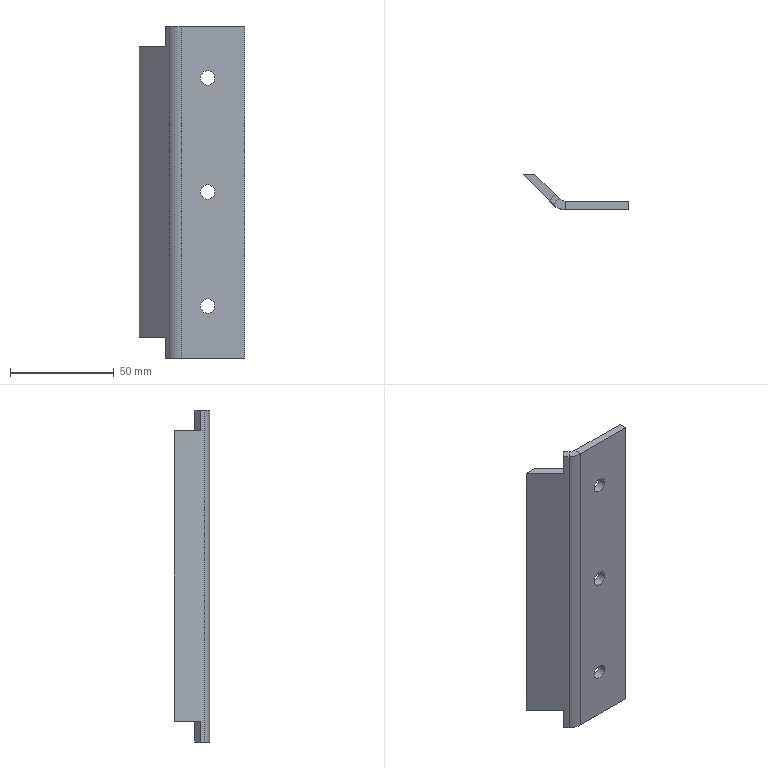Part | SolidWorks | 1 solid | 24 faces | box 51.059 x 17.007 x 160 mm | volume 32939 mm3 | plane 16 | cylinder 8 | commonest cylinder face diameters 7 x6 8 x1 16 x1
STEP:
#1=CARTESIAN_POINT('',(18.5,4.,55.));
#2=VERTEX_POINT('',#1);
#3=CARTESIAN_POINT('',(18.5,0.,55.));
#4=VERTEX_POINT('',#3);
#5=CARTESIAN_POINT('',(18.5,4.,55.));
#6=DIRECTION('',(0.,-1.,0.));
#7=VECTOR('',#6,1000.);
#8=LINE('',#5,#7);
#9=EDGE_CURVE('',#2,#4,#8,.T.);
#10=ORIENTED_EDGE('',*,*,#9,.F.);
#11=CARTESIAN_POINT('',(11.5,4.,55.));
#12=VERTEX_POINT('',#11);
#13=CARTESIAN_POINT('',(15.,4.,55.));
#14=DIRECTION('',(0.,1.,0.));
#15=DIRECTION('',(1.,0.,0.));
#16=AXIS2_PLACEMENT_3D('',#13,#14,#15);
#17=CIRCLE('',#16,3.5);
#18=EDGE_CURVE('',#2,#12,#17,.T.);
#19=ORIENTED_EDGE('',*,*,#18,.T.);
#20=CARTESIAN_POINT('',(11.5,0.,55.));
#21=VERTEX_POINT('',#20);
#22=CARTESIAN_POINT('',(11.5,4.,55.));
#23=DIRECTION('',(0.,-1.,0.));
#24=VECTOR('',#23,1000.);
#25=LINE('',#22,#24);
#26=EDGE_CURVE('',#12,#21,#25,.T.);
#27=ORIENTED_EDGE('',*,*,#26,.T.);
#28=CARTESIAN_POINT('',(15.,0.,55.));
#29=DIRECTION('',(0.,-1.,0.));
#30=DIRECTION('',(-1.,0.,0.));
#31=AXIS2_PLACEMENT_3D('',#28,#29,#30);
#32=CIRCLE('',#31,3.5);
#33=EDGE_CURVE('',#21,#4,#32,.T.);
#34=ORIENTED_EDGE('',*,*,#33,.T.);
#35=EDGE_LOOP('',(#10,#19,#27,#34));
#36=FACE_OUTER_BOUND('',#35,.T.);
#37=CARTESIAN_POINT('',(15.,2.,55.));
#38=DIRECTION('',(0.,1.,0.));
#39=DIRECTION('',(1.,0.,0.));
#40=AXIS2_PLACEMENT_3D('',#37,#38,#39);
#41=CYLINDRICAL_SURFACE('',#40,3.5);
#42=ADVANCED_FACE('',(#36),#41,.F.);
#43=CARTESIAN_POINT('',(15.,4.,55.));
#44=DIRECTION('',(0.,1.,0.));
#45=DIRECTION('',(-1.,0.,0.));
#46=AXIS2_PLACEMENT_3D('',#43,#44,#45);
#47=CIRCLE('',#46,3.5);
#48=EDGE_CURVE('',#12,#2,#47,.T.);
#49=ORIENTED_EDGE('',*,*,#48,.T.);
#50=ORIENTED_EDGE('',*,*,#9,.T.);
#51=CARTESIAN_POINT('',(15.,0.,55.));
#52=DIRECTION('',(0.,-1.,0.));
#53=DIRECTION('',(1.,0.,0.));
#54=AXIS2_PLACEMENT_3D('',#51,#52,#53);
#55=CIRCLE('',#54,3.5);
#56=EDGE_CURVE('',#4,#21,#55,.T.);
#57=ORIENTED_EDGE('',*,*,#56,.T.);
#58=ORIENTED_EDGE('',*,*,#26,.F.);
#59=EDGE_LOOP('',(#49,#50,#57,#58));
#60=FACE_OUTER_BOUND('',#59,.T.);
#61=CARTESIAN_POINT('',(15.,2.,55.));
#62=DIRECTION('',(0.,1.,0.));
#63=DIRECTION('',(1.,0.,0.));
#64=AXIS2_PLACEMENT_3D('',#61,#62,#63);
#65=CYLINDRICAL_SURFACE('',#64,3.5);
#66=ADVANCED_FACE('',(#60),#65,.F.);
#67=CARTESIAN_POINT('',(18.5,4.,-55.));
#68=VERTEX_POINT('',#67);
#69=CARTESIAN_POINT('',(18.5,0.,-55.));
#70=VERTEX_POINT('',#69);
#71=CARTESIAN_POINT('',(18.5,4.,-55.));
#72=DIRECTION('',(0.,-1.,0.));
#73=VECTOR('',#72,1000.);
#74=LINE('',#71,#73);
#75=EDGE_CURVE('',#68,#70,#74,.T.);
#76=ORIENTED_EDGE('',*,*,#75,.F.);
#77=CARTESIAN_POINT('',(11.5,4.,-55.));
#78=VERTEX_POINT('',#77);
#79=CARTESIAN_POINT('',(15.,4.,-55.));
#80=DIRECTION('',(0.,1.,0.));
#81=DIRECTION('',(1.,0.,0.));
#82=AXIS2_PLACEMENT_3D('',#79,#80,#81);
#83=CIRCLE('',#82,3.5);
#84=EDGE_CURVE('',#68,#78,#83,.T.);
#85=ORIENTED_EDGE('',*,*,#84,.T.);
#86=CARTESIAN_POINT('',(11.5,0.,-55.));
#87=VERTEX_POINT('',#86);
#88=CARTESIAN_POINT('',(11.5,4.,-55.));
#89=DIRECTION('',(0.,-1.,0.));
#90=VECTOR('',#89,1000.);
#91=LINE('',#88,#90);
#92=EDGE_CURVE('',#78,#87,#91,.T.);
#93=ORIENTED_EDGE('',*,*,#92,.T.);
#94=CARTESIAN_POINT('',(15.,0.,-55.));
#95=DIRECTION('',(0.,-1.,0.));
#96=DIRECTION('',(-1.,0.,0.));
#97=AXIS2_PLACEMENT_3D('',#94,#95,#96);
#98=CIRCLE('',#97,3.5);
#99=EDGE_CURVE('',#87,#70,#98,.T.);
#100=ORIENTED_EDGE('',*,*,#99,.T.);
#101=EDGE_LOOP('',(#76,#85,#93,#100));
#102=FACE_OUTER_BOUND('',#101,.T.);
#103=CARTESIAN_POINT('',(15.,2.,-55.));
#104=DIRECTION('',(0.,1.,0.));
#105=DIRECTION('',(1.,0.,0.));
#106=AXIS2_PLACEMENT_3D('',#103,#104,#105);
#107=CYLINDRICAL_SURFACE('',#106,3.5);
#108=ADVANCED_FACE('',(#102),#107,.F.);
#109=CARTESIAN_POINT('',(15.,4.,-55.));
#110=DIRECTION('',(0.,1.,0.));
#111=DIRECTION('',(-1.,0.,0.));
#112=AXIS2_PLACEMENT_3D('',#109,#110,#111);
#113=CIRCLE('',#112,3.5);
#114=EDGE_CURVE('',#78,#68,#113,.T.);
#115=ORIENTED_EDGE('',*,*,#114,.T.);
#116=ORIENTED_EDGE('',*,*,#75,.T.);
#117=CARTESIAN_POINT('',(15.,0.,-55.));
#118=DIRECTION('',(0.,-1.,0.));
#119=DIRECTION('',(1.,0.,0.));
#120=AXIS2_PLACEMENT_3D('',#117,#118,#119);
#121=CIRCLE('',#120,3.5);
#122=EDGE_CURVE('',#70,#87,#121,.T.);
#123=ORIENTED_EDGE('',*,*,#122,.T.);
#124=ORIENTED_EDGE('',*,*,#92,.F.);
#125=EDGE_LOOP('',(#115,#116,#123,#124));
#126=FACE_OUTER_BOUND('',#125,.T.);
#127=CARTESIAN_POINT('',(15.,2.,-55.));
#128=DIRECTION('',(0.,1.,0.));
#129=DIRECTION('',(1.,0.,0.));
#130=AXIS2_PLACEMENT_3D('',#127,#128,#129);
#131=CYLINDRICAL_SURFACE('',#130,3.5);
#132=ADVANCED_FACE('',(#126),#131,.F.);
#133=CARTESIAN_POINT('',(18.5,4.,0.));
#134=VERTEX_POINT('',#133);
#135=CARTESIAN_POINT('',(18.5,0.,0.));
#136=VERTEX_POINT('',#135);
#137=CARTESIAN_POINT('',(18.5,4.,0.));
#138=DIRECTION('',(0.,-1.,0.));
#139=VECTOR('',#138,1000.);
#140=LINE('',#137,#139);
#141=EDGE_CURVE('',#134,#136,#140,.T.);
#142=ORIENTED_EDGE('',*,*,#141,.F.);
#143=CARTESIAN_POINT('',(11.5,4.,0.));
#144=VERTEX_POINT('',#143);
#145=CARTESIAN_POINT('',(15.,4.,0.));
#146=DIRECTION('',(0.,1.,0.));
#147=DIRECTION('',(1.,0.,0.));
#148=AXIS2_PLACEMENT_3D('',#145,#146,#147);
#149=CIRCLE('',#148,3.5);
#150=EDGE_CURVE('',#134,#144,#149,.T.);
#151=ORIENTED_EDGE('',*,*,#150,.T.);
#152=CARTESIAN_POINT('',(11.5,0.,0.));
#153=VERTEX_POINT('',#152);
#154=CARTESIAN_POINT('',(11.5,4.,0.));
#155=DIRECTION('',(0.,-1.,0.));
#156=VECTOR('',#155,1000.);
#157=LINE('',#154,#156);
#158=EDGE_CURVE('',#144,#153,#157,.T.);
#159=ORIENTED_EDGE('',*,*,#158,.T.);
#160=CARTESIAN_POINT('',(15.,0.,0.));
#161=DIRECTION('',(0.,-1.,0.));
#162=DIRECTION('',(-1.,0.,0.));
#163=AXIS2_PLACEMENT_3D('',#160,#161,#162);
#164=CIRCLE('',#163,3.5);
#165=EDGE_CURVE('',#153,#136,#164,.T.);
#166=ORIENTED_EDGE('',*,*,#165,.T.);
#167=EDGE_LOOP('',(#142,#151,#159,#166));
#168=FACE_OUTER_BOUND('',#167,.T.);
#169=CARTESIAN_POINT('',(15.,2.,0.));
#170=DIRECTION('',(0.,1.,0.));
#171=DIRECTION('',(1.,0.,0.));
#172=AXIS2_PLACEMENT_3D('',#169,#170,#171);
#173=CYLINDRICAL_SURFACE('',#172,3.5);
#174=ADVANCED_FACE('',(#168),#173,.F.);
#175=CARTESIAN_POINT('',(15.,4.,0.));
#176=DIRECTION('',(0.,1.,0.));
#177=DIRECTION('',(-1.,0.,0.));
#178=AXIS2_PLACEMENT_3D('',#175,#176,#177);
#179=CIRCLE('',#178,3.5);
#180=EDGE_CURVE('',#144,#134,#179,.T.);
#181=ORIENTED_EDGE('',*,*,#180,.T.);
#182=ORIENTED_EDGE('',*,*,#141,.T.);
#183=CARTESIAN_POINT('',(15.,0.,0.));
#184=DIRECTION('',(0.,-1.,0.));
#185=DIRECTION('',(1.,0.,0.));
#186=AXIS2_PLACEMENT_3D('',#183,#184,#185);
#187=CIRCLE('',#186,3.5);
#188=EDGE_CURVE('',#136,#153,#187,.T.);
#189=ORIENTED_EDGE('',*,*,#188,.T.);
#190=ORIENTED_EDGE('',*,*,#158,.F.);
#191=EDGE_LOOP('',(#181,#182,#189,#190));
#192=FACE_OUTER_BOUND('',#191,.T.);
#193=CARTESIAN_POINT('',(15.,2.,0.));
#194=DIRECTION('',(0.,1.,0.));
#195=DIRECTION('',(1.,0.,0.));
#196=AXIS2_PLACEMENT_3D('',#193,#194,#195);
#197=CYLINDRICAL_SURFACE('',#196,3.5);
#198=ADVANCED_FACE('',(#192),#197,.F.);
#199=CARTESIAN_POINT('',(33.,4.,-80.));
#200=VERTEX_POINT('',#199);
#201=CARTESIAN_POINT('',(33.,4.,80.));
#202=VERTEX_POINT('',#201);
#203=CARTESIAN_POINT('',(33.,4.,-80.));
#204=DIRECTION('',(0.,0.,1.));
#205=VECTOR('',#204,1000.);
#206=LINE('',#203,#205);
#207=EDGE_CURVE('',#200,#202,#206,.T.);
#208=ORIENTED_EDGE('',*,*,#207,.T.);
#209=CARTESIAN_POINT('',(33.,0.,80.));
#210=VERTEX_POINT('',#209);
#211=CARTESIAN_POINT('',(33.,0.,80.));
#212=DIRECTION('',(0.,1.,0.));
#213=VECTOR('',#212,1000.);
#214=LINE('',#211,#213);
#215=EDGE_CURVE('',#210,#202,#214,.T.);
#216=ORIENTED_EDGE('',*,*,#215,.F.);
#217=CARTESIAN_POINT('',(33.,0.,-80.));
#218=VERTEX_POINT('',#217);
#219=CARTESIAN_POINT('',(33.,0.,-80.));
#220=DIRECTION('',(0.,0.,1.));
#221=VECTOR('',#220,1000.);
#222=LINE('',#219,#221);
#223=EDGE_CURVE('',#218,#210,#222,.T.);
#224=ORIENTED_EDGE('',*,*,#223,.F.);
#225=CARTESIAN_POINT('',(33.,0.,-80.));
#226=DIRECTION('',(0.,1.,0.));
#227=VECTOR('',#226,1000.);
#228=LINE('',#225,#227);
#229=EDGE_CURVE('',#218,#200,#228,.T.);
#230=ORIENTED_EDGE('',*,*,#229,.T.);
#231=EDGE_LOOP('',(#208,#216,#224,#230));
#232=FACE_OUTER_BOUND('',#231,.T.);
#233=CARTESIAN_POINT('',(33.,4.,80.));
#234=DIRECTION('',(1.,0.,0.));
#235=DIRECTION('',(0.,1.,0.));
#236=AXIS2_PLACEMENT_3D('',#233,#234,#235);
#237=PLANE('',#236);
#238=ADVANCED_FACE('',(#232),#237,.T.);
#239=CARTESIAN_POINT('',(-2.503,7.108,70.));
#240=VERTEX_POINT('',#239);
#241=CARTESIAN_POINT('',(-5.331,4.279,70.));
#242=VERTEX_POINT('',#241);
#243=CARTESIAN_POINT('',(-2.503,7.108,70.));
#244=DIRECTION('',(-0.7071,-0.7071,0.));
#245=VECTOR('',#244,1000.);
#246=LINE('',#243,#245);
#247=EDGE_CURVE('',#240,#242,#246,.T.);
#248=ORIENTED_EDGE('',*,*,#247,.F.);
#249=CARTESIAN_POINT('',(-12.402,17.007,70.));
#250=VERTEX_POINT('',#249);
#251=CARTESIAN_POINT('',(-12.402,17.007,70.));
#252=DIRECTION('',(0.7071,-0.7071,0.));
#253=VECTOR('',#252,1000.);
#254=LINE('',#251,#253);
#255=EDGE_CURVE('',#250,#240,#254,.T.);
#256=ORIENTED_EDGE('',*,*,#255,.F.);
#257=CARTESIAN_POINT('',(-18.059,17.007,70.));
#258=VERTEX_POINT('',#257);
#259=CARTESIAN_POINT('',(-12.402,17.007,70.));
#260=DIRECTION('',(-1.,0.,0.));
#261=VECTOR('',#260,1000.);
#262=LINE('',#259,#261);
#263=EDGE_CURVE('',#250,#258,#262,.T.);
#264=ORIENTED_EDGE('',*,*,#263,.T.);
#265=CARTESIAN_POINT('',(-5.331,4.279,70.));
#266=DIRECTION('',(-0.7071,0.7071,0.));
#267=VECTOR('',#266,1000.);
#268=LINE('',#265,#267);
#269=EDGE_CURVE('',#242,#258,#268,.T.);
#270=ORIENTED_EDGE('',*,*,#269,.F.);
#271=EDGE_LOOP('',(#248,#256,#264,#270));
#272=FACE_OUTER_BOUND('',#271,.T.);
#273=CARTESIAN_POINT('',(-15.23,19.836,70.));
#274=DIRECTION('',(0.,0.,-1.));
#275=DIRECTION('',(0.,-1.,0.));
#276=AXIS2_PLACEMENT_3D('',#273,#274,#275);
#277=PLANE('',#276);
#278=ADVANCED_FACE('',(#272),#277,.F.);
#279=CARTESIAN_POINT('',(-5.331,4.279,80.));
#280=VERTEX_POINT('',#279);
#281=CARTESIAN_POINT('',(-5.331,4.279,70.));
#282=DIRECTION('',(0.,0.,1.));
#283=VECTOR('',#282,1000.);
#284=LINE('',#281,#283);
#285=EDGE_CURVE('',#242,#280,#284,.T.);
#286=ORIENTED_EDGE('',*,*,#285,.T.);
#287=CARTESIAN_POINT('',(-2.503,7.108,80.));
#288=VERTEX_POINT('',#287);
#289=CARTESIAN_POINT('',(-5.331,4.279,80.));
#290=DIRECTION('',(0.7071,0.7071,0.));
#291=VECTOR('',#290,1000.);
#292=LINE('',#289,#291);
#293=EDGE_CURVE('',#280,#288,#292,.T.);
#294=ORIENTED_EDGE('',*,*,#293,.T.);
#295=CARTESIAN_POINT('',(-2.503,7.108,80.));
#296=DIRECTION('',(0.,0.,-1.));
#297=VECTOR('',#296,1000.);
#298=LINE('',#295,#297);
#299=EDGE_CURVE('',#288,#240,#298,.T.);
#300=ORIENTED_EDGE('',*,*,#299,.T.);
#301=ORIENTED_EDGE('',*,*,#247,.T.);
#302=EDGE_LOOP('',(#286,#294,#300,#301));
#303=FACE_OUTER_BOUND('',#302,.T.);
#304=CARTESIAN_POINT('',(-2.503,7.108,70.));
#305=DIRECTION('',(0.7071,-0.7071,0.));
#306=DIRECTION('',(0.,0.,-1.));
#307=AXIS2_PLACEMENT_3D('',#304,#305,#306);
#308=PLANE('',#307);
#309=ADVANCED_FACE('',(#303),#308,.F.);
#310=CARTESIAN_POINT('',(-3.395,2.343,-80.));
#311=VERTEX_POINT('',#310);
#312=CARTESIAN_POINT('',(2.262,0.,-80.));
#313=VERTEX_POINT('',#312);
#314=CARTESIAN_POINT('',(2.262,8.,-80.));
#315=DIRECTION('',(0.,0.,1.));
#316=DIRECTION('',(-0.7071,-0.7071,0.));
#317=AXIS2_PLACEMENT_3D('',#314,#315,#316);
#318=CIRCLE('',#317,8.);
#319=EDGE_CURVE('',#311,#313,#318,.T.);
#320=ORIENTED_EDGE('',*,*,#319,.T.);
#321=CARTESIAN_POINT('',(2.262,0.,80.));
#322=VERTEX_POINT('',#321);
#323=CARTESIAN_POINT('',(2.262,0.,80.));
#324=DIRECTION('',(0.,0.,-1.));
#325=VECTOR('',#324,1000.);
#326=LINE('',#323,#325);
#327=EDGE_CURVE('',#322,#313,#326,.T.);
#328=ORIENTED_EDGE('',*,*,#327,.F.);
#329=CARTESIAN_POINT('',(-3.395,2.343,80.));
#330=VERTEX_POINT('',#329);
#331=CARTESIAN_POINT('',(2.262,8.,80.));
#332=DIRECTION('',(0.,0.,-1.));
#333=DIRECTION('',(0.,-1.,0.));
#334=AXIS2_PLACEMENT_3D('',#331,#332,#333);
#335=CIRCLE('',#334,8.);
#336=EDGE_CURVE('',#322,#330,#335,.T.);
#337=ORIENTED_EDGE('',*,*,#336,.T.);
#338=CARTESIAN_POINT('',(-3.395,2.343,-80.));
#339=DIRECTION('',(0.,0.,1.));
#340=VECTOR('',#339,1000.);
#341=LINE('',#338,#340);
#342=EDGE_CURVE('',#311,#330,#341,.T.);
#343=ORIENTED_EDGE('',*,*,#342,.F.);
#344=EDGE_LOOP('',(#320,#328,#337,#343));
#345=FACE_OUTER_BOUND('',#344,.T.);
#346=CARTESIAN_POINT('',(2.262,8.,0.));
#347=DIRECTION('',(0.,0.,-1.));
#348=DIRECTION('',(0.,-1.,0.));
#349=AXIS2_PLACEMENT_3D('',#346,#347,#348);
#350=CYLINDRICAL_SURFACE('',#349,8.);
#351=ADVANCED_FACE('',(#345),#350,.T.);
#352=CARTESIAN_POINT('',(-0.5665,5.172,80.));
#353=VERTEX_POINT('',#352);
#354=CARTESIAN_POINT('',(2.262,4.,80.));
#355=VERTEX_POINT('',#354);
#356=CARTESIAN_POINT('',(2.262,8.,80.));
#357=DIRECTION('',(0.,0.,1.));
#358=DIRECTION('',(-0.7071,-0.7071,0.));
#359=AXIS2_PLACEMENT_3D('',#356,#357,#358);
#360=CIRCLE('',#359,4.);
#361=EDGE_CURVE('',#353,#355,#360,.T.);
#362=ORIENTED_EDGE('',*,*,#361,.F.);
#363=CARTESIAN_POINT('',(-0.5665,5.172,80.));
#364=DIRECTION('',(-0.7071,-0.7071,0.));
#365=VECTOR('',#364,1000.);
#366=LINE('',#363,#365);
#367=EDGE_CURVE('',#353,#330,#366,.T.);
#368=ORIENTED_EDGE('',*,*,#367,.T.);
#369=ORIENTED_EDGE('',*,*,#336,.F.);
#370=CARTESIAN_POINT('',(2.262,0.,80.));
#371=DIRECTION('',(0.,1.,0.));
#372=VECTOR('',#371,1000.);
#373=LINE('',#370,#372);
#374=EDGE_CURVE('',#322,#355,#373,.T.);
#375=ORIENTED_EDGE('',*,*,#374,.T.);
#376=EDGE_LOOP('',(#362,#368,#369,#375));
#377=FACE_OUTER_BOUND('',#376,.T.);
#378=CARTESIAN_POINT('',(2.262,-7.,80.));
#379=DIRECTION('',(0.,0.,-1.));
#380=DIRECTION('',(0.,-1.,0.));
#381=AXIS2_PLACEMENT_3D('',#378,#379,#380);
#382=PLANE('',#381);
#383=ADVANCED_FACE('',(#377),#382,.F.);
#384=ORIENTED_EDGE('',*,*,#293,.F.);
#385=CARTESIAN_POINT('',(-3.395,2.343,80.));
#386=DIRECTION('',(-0.7071,0.7071,0.));
#387=VECTOR('',#386,1000.);
#388=LINE('',#385,#387);
#389=EDGE_CURVE('',#330,#280,#388,.T.);
#390=ORIENTED_EDGE('',*,*,#389,.F.);
#391=ORIENTED_EDGE('',*,*,#367,.F.);
#392=CARTESIAN_POINT('',(-2.503,7.108,80.));
#393=DIRECTION('',(0.7071,-0.7071,0.));
#394=VECTOR('',#393,1000.);
#395=LINE('',#392,#394);
#396=EDGE_CURVE('',#288,#353,#395,.T.);
#397=ORIENTED_EDGE('',*,*,#396,.F.);
#398=EDGE_LOOP('',(#384,#390,#391,#397));
#399=FACE_OUTER_BOUND('',#398,.T.);
#400=CARTESIAN_POINT('',(14.468,-15.52,80.));
#401=DIRECTION('',(0.,0.,1.));
#402=DIRECTION('',(1.,0.,0.));
#403=AXIS2_PLACEMENT_3D('',#400,#401,#402);
#404=PLANE('',#403);
#405=ADVANCED_FACE('',(#399),#404,.T.);
#406=CARTESIAN_POINT('',(-5.331,4.279,-80.));
#407=VERTEX_POINT('',#406);
#408=CARTESIAN_POINT('',(-5.331,4.279,-70.));
#409=VERTEX_POINT('',#408);
#410=CARTESIAN_POINT('',(-5.331,4.279,-80.));
#411=DIRECTION('',(0.,0.,1.));
#412=VECTOR('',#411,1000.);
#413=LINE('',#410,#412);
#414=EDGE_CURVE('',#407,#409,#413,.T.);
#415=ORIENTED_EDGE('',*,*,#414,.T.);
#416=CARTESIAN_POINT('',(-2.503,7.108,-70.));
#417=VERTEX_POINT('',#416);
#418=CARTESIAN_POINT('',(-5.331,4.279,-70.));
#419=DIRECTION('',(0.7071,0.7071,0.));
#420=VECTOR('',#419,1000.);
#421=LINE('',#418,#420);
#422=EDGE_CURVE('',#409,#417,#421,.T.);
#423=ORIENTED_EDGE('',*,*,#422,.T.);
#424=CARTESIAN_POINT('',(-2.503,7.108,-80.));
#425=VERTEX_POINT('',#424);
#426=CARTESIAN_POINT('',(-2.503,7.108,-70.));
#427=DIRECTION('',(0.,0.,-1.));
#428=VECTOR('',#427,1000.);
#429=LINE('',#426,#428);
#430=EDGE_CURVE('',#417,#425,#429,.T.);
#431=ORIENTED_EDGE('',*,*,#430,.T.);
#432=CARTESIAN_POINT('',(-2.503,7.108,-80.));
#433=DIRECTION('',(-0.7071,-0.7071,0.));
#434=VECTOR('',#433,1000.);
#435=LINE('',#432,#434);
#436=EDGE_CURVE('',#425,#407,#435,.T.);
#437=ORIENTED_EDGE('',*,*,#436,.T.);
#438=EDGE_LOOP('',(#415,#423,#431,#437));
#439=FACE_OUTER_BOUND('',#438,.T.);
#440=CARTESIAN_POINT('',(-2.503,7.108,-80.));
#441=DIRECTION('',(0.7071,-0.7071,0.));
#442=DIRECTION('',(0.,0.,-1.));
#443=AXIS2_PLACEMENT_3D('',#440,#441,#442);
#444=PLANE('',#443);
#445=ADVANCED_FACE('',(#439),#444,.F.);
#446=ORIENTED_EDGE('',*,*,#255,.T.);
#447=ORIENTED_EDGE('',*,*,#299,.F.);
#448=ORIENTED_EDGE('',*,*,#396,.T.);
#449=CARTESIAN_POINT('',(-0.5665,5.172,-80.));
#450=VERTEX_POINT('',#449);
#451=CARTESIAN_POINT('',(-0.5665,5.172,80.));
#452=DIRECTION('',(0.,0.,-1.));
#453=VECTOR('',#452,1000.);
#454=LINE('',#451,#453);
#455=EDGE_CURVE('',#353,#450,#454,.T.);
#456=ORIENTED_EDGE('',*,*,#455,.T.);
#457=CARTESIAN_POINT('',(-0.5665,5.172,-80.));
#458=DIRECTION('',(-0.7071,0.7071,0.));
#459=VECTOR('',#458,1000.);
#460=LINE('',#457,#459);
#461=EDGE_CURVE('',#450,#425,#460,.T.);
#462=ORIENTED_EDGE('',*,*,#461,.T.);
#463=ORIENTED_EDGE('',*,*,#430,.F.);
#464=CARTESIAN_POINT('',(-12.402,17.007,-70.));
#465=VERTEX_POINT('',#464);
#466=CARTESIAN_POINT('',(-2.503,7.108,-70.));
#467=DIRECTION('',(-0.7071,0.7071,0.));
#468=VECTOR('',#467,1000.);
#469=LINE('',#466,#468);
#470=EDGE_CURVE('',#417,#465,#469,.T.);
#471=ORIENTED_EDGE('',*,*,#470,.T.);
#472=CARTESIAN_POINT('',(-12.402,17.007,-70.));
#473=DIRECTION('',(0.,0.,1.));
#474=VECTOR('',#473,1000.);
#475=LINE('',#472,#474);
#476=EDGE_CURVE('',#465,#250,#475,.T.);
#477=ORIENTED_EDGE('',*,*,#476,.T.);
#478=EDGE_LOOP('',(#446,#447,#448,#456,#462,#463,#471,#477));
#479=FACE_OUTER_BOUND('',#478,.T.);
#480=CARTESIAN_POINT('',(1.033,3.572,0.));
#481=DIRECTION('',(0.7071,0.7071,0.));
#482=DIRECTION('',(0.,0.,-1.));
#483=AXIS2_PLACEMENT_3D('',#480,#481,#482);
#484=PLANE('',#483);
#485=ADVANCED_FACE('',(#479),#484,.T.);
#486=ORIENTED_EDGE('',*,*,#422,.F.);
#487=CARTESIAN_POINT('',(-18.059,17.007,-70.));
#488=VERTEX_POINT('',#487);
#489=CARTESIAN_POINT('',(-18.059,17.007,-70.));
#490=DIRECTION('',(0.7071,-0.7071,0.));
#491=VECTOR('',#490,1000.);
#492=LINE('',#489,#491);
#493=EDGE_CURVE('',#488,#409,#492,.T.);
#494=ORIENTED_EDGE('',*,*,#493,.F.);
#495=CARTESIAN_POINT('',(-18.059,17.007,-70.));
#496=DIRECTION('',(1.,0.,0.));
#497=VECTOR('',#496,1000.);
#498=LINE('',#495,#497);
#499=EDGE_CURVE('',#488,#465,#498,.T.);
#500=ORIENTED_EDGE('',*,*,#499,.T.);
#501=ORIENTED_EDGE('',*,*,#470,.F.);
#502=EDGE_LOOP('',(#486,#494,#500,#501));
#503=FACE_OUTER_BOUND('',#502,.T.);
#504=CARTESIAN_POINT('',(-2.503,7.108,-70.));
#505=DIRECTION('',(0.,0.,1.));
#506=DIRECTION('',(1.,0.,0.));
#507=AXIS2_PLACEMENT_3D('',#504,#505,#506);
#508=PLANE('',#507);
#509=ADVANCED_FACE('',(#503),#508,.F.);
#510=ORIENTED_EDGE('',*,*,#263,.F.);
#511=ORIENTED_EDGE('',*,*,#476,.F.);
#512=ORIENTED_EDGE('',*,*,#499,.F.);
#513=CARTESIAN_POINT('',(-18.059,17.007,70.));
#514=DIRECTION('',(0.,0.,-1.));
#515=VECTOR('',#514,1000.);
#516=LINE('',#513,#515);
#517=EDGE_CURVE('',#258,#488,#516,.T.);
#518=ORIENTED_EDGE('',*,*,#517,.F.);
#519=EDGE_LOOP('',(#510,#511,#512,#518));
#520=FACE_OUTER_BOUND('',#519,.T.);
#521=CARTESIAN_POINT('',(-15.23,17.007,40.));
#522=DIRECTION('',(0.,1.,0.));
#523=DIRECTION('',(1.,0.,0.));
#524=AXIS2_PLACEMENT_3D('',#521,#522,#523);
#525=PLANE('',#524);
#526=ADVANCED_FACE('',(#520),#525,.T.);
#527=ORIENTED_EDGE('',*,*,#493,.T.);
#528=ORIENTED_EDGE('',*,*,#414,.F.);
#529=CARTESIAN_POINT('',(-5.331,4.279,-80.));
#530=DIRECTION('',(0.7071,-0.7071,0.));
#531=VECTOR('',#530,1000.);
#532=LINE('',#529,#531);
#533=EDGE_CURVE('',#407,#311,#532,.T.);
#534=ORIENTED_EDGE('',*,*,#533,.T.);
#535=ORIENTED_EDGE('',*,*,#342,.T.);
#536=ORIENTED_EDGE('',*,*,#389,.T.);
#537=ORIENTED_EDGE('',*,*,#285,.F.);
#538=ORIENTED_EDGE('',*,*,#269,.T.);
#539=ORIENTED_EDGE('',*,*,#517,.T.);
#540=EDGE_LOOP('',(#527,#528,#534,#535,#536,#537,#538,#539));
#541=FACE_OUTER_BOUND('',#540,.T.);
#542=CARTESIAN_POINT('',(-1.795,0.7437,0.));
#543=DIRECTION('',(0.7071,0.7071,0.));
#544=DIRECTION('',(0.,0.,-1.));
#545=AXIS2_PLACEMENT_3D('',#542,#543,#544);
#546=PLANE('',#545);
#547=ADVANCED_FACE('',(#541),#546,.F.);
#548=ORIENTED_EDGE('',*,*,#436,.F.);
#549=ORIENTED_EDGE('',*,*,#461,.F.);
#550=CARTESIAN_POINT('',(-3.395,2.343,-80.));
#551=DIRECTION('',(0.7071,0.7071,0.));
#552=VECTOR('',#551,1000.);
#553=LINE('',#550,#552);
#554=EDGE_CURVE('',#311,#450,#553,.T.);
#555=ORIENTED_EDGE('',*,*,#554,.F.);
#556=ORIENTED_EDGE('',*,*,#533,.F.);
#557=EDGE_LOOP('',(#548,#549,#555,#556));
#558=FACE_OUTER_BOUND('',#557,.T.);
#559=CARTESIAN_POINT('',(-18.059,17.007,-80.));
#560=DIRECTION('',(0.,0.,-1.));
#561=DIRECTION('',(0.,-1.,0.));
#562=AXIS2_PLACEMENT_3D('',#559,#560,#561);
#563=PLANE('',#562);
#564=ADVANCED_FACE('',(#558),#563,.T.);
#565=CARTESIAN_POINT('',(2.262,4.,-80.));
#566=VERTEX_POINT('',#565);
#567=CARTESIAN_POINT('',(2.262,8.,-80.));
#568=DIRECTION('',(0.,0.,-1.));
#569=DIRECTION('',(0.,-1.,0.));
#570=AXIS2_PLACEMENT_3D('',#567,#568,#569);
#571=CIRCLE('',#570,4.);
#572=EDGE_CURVE('',#566,#450,#571,.T.);
#573=ORIENTED_EDGE('',*,*,#572,.F.);
#574=CARTESIAN_POINT('',(2.262,4.,-80.));
#575=DIRECTION('',(0.,-1.,0.));
#576=VECTOR('',#575,1000.);
#577=LINE('',#574,#576);
#578=EDGE_CURVE('',#566,#313,#577,.T.);
#579=ORIENTED_EDGE('',*,*,#578,.T.);
#580=ORIENTED_EDGE('',*,*,#319,.F.);
#581=ORIENTED_EDGE('',*,*,#554,.T.);
#582=EDGE_LOOP('',(#573,#579,#580,#581));
#583=FACE_OUTER_BOUND('',#582,.T.);
#584=CARTESIAN_POINT('',(2.262,-7.,-80.));
#585=DIRECTION('',(0.,0.,-1.));
#586=DIRECTION('',(0.,-1.,0.));
#587=AXIS2_PLACEMENT_3D('',#584,#585,#586);
#588=PLANE('',#587);
#589=ADVANCED_FACE('',(#583),#588,.T.);
#590=ORIENTED_EDGE('',*,*,#229,.F.);
#591=CARTESIAN_POINT('',(33.,0.,-80.));
#592=DIRECTION('',(-1.,0.,0.));
#593=VECTOR('',#592,1000.);
#594=LINE('',#591,#593);
#595=EDGE_CURVE('',#218,#313,#594,.T.);
#596=ORIENTED_EDGE('',*,*,#595,.T.);
#597=ORIENTED_EDGE('',*,*,#578,.F.);
#598=CARTESIAN_POINT('',(2.262,4.,-80.));
#599=DIRECTION('',(1.,0.,0.));
#600=VECTOR('',#599,1000.);
#601=LINE('',#598,#600);
#602=EDGE_CURVE('',#566,#200,#601,.T.);
#603=ORIENTED_EDGE('',*,*,#602,.T.);
#604=EDGE_LOOP('',(#590,#596,#597,#603));
#605=FACE_OUTER_BOUND('',#604,.T.);
#606=CARTESIAN_POINT('',(-23.,0.,-80.));
#607=DIRECTION('',(0.,0.,-1.));
#608=DIRECTION('',(0.,-1.,0.));
#609=AXIS2_PLACEMENT_3D('',#606,#607,#608);
#610=PLANE('',#609);
#611=ADVANCED_FACE('',(#605),#610,.T.);
#612=ORIENTED_EDGE('',*,*,#33,.F.);
#613=ORIENTED_EDGE('',*,*,#56,.F.);
#614=EDGE_LOOP('',(#612,#613));
#615=FACE_BOUND('',#614,.T.);
#616=ORIENTED_EDGE('',*,*,#99,.F.);
#617=ORIENTED_EDGE('',*,*,#122,.F.);
#618=EDGE_LOOP('',(#616,#617));
#619=FACE_BOUND('',#618,.T.);
#620=ORIENTED_EDGE('',*,*,#165,.F.);
#621=ORIENTED_EDGE('',*,*,#188,.F.);
#622=EDGE_LOOP('',(#620,#621));
#623=FACE_BOUND('',#622,.T.);
#624=ORIENTED_EDGE('',*,*,#223,.T.);
#625=CARTESIAN_POINT('',(2.262,0.,80.));
#626=DIRECTION('',(1.,0.,0.));
#627=VECTOR('',#626,1000.);
#628=LINE('',#625,#627);
#629=EDGE_CURVE('',#322,#210,#628,.T.);
#630=ORIENTED_EDGE('',*,*,#629,.F.);
#631=ORIENTED_EDGE('',*,*,#327,.T.);
#632=ORIENTED_EDGE('',*,*,#595,.F.);
#633=EDGE_LOOP('',(#624,#630,#631,#632));
#634=FACE_OUTER_BOUND('',#633,.T.);
#635=CARTESIAN_POINT('',(0.,0.,0.));
#636=DIRECTION('',(0.,1.,0.));
#637=DIRECTION('',(1.,0.,0.));
#638=AXIS2_PLACEMENT_3D('',#635,#636,#637);
#639=PLANE('',#638);
#640=ADVANCED_FACE('',(#615,#619,#623,#634),#639,.F.);
#641=ORIENTED_EDGE('',*,*,#215,.T.);
#642=CARTESIAN_POINT('',(2.262,4.,80.));
#643=DIRECTION('',(1.,0.,0.));
#644=VECTOR('',#643,1000.);
#645=LINE('',#642,#644);
#646=EDGE_CURVE('',#355,#202,#645,.T.);
#647=ORIENTED_EDGE('',*,*,#646,.F.);
#648=ORIENTED_EDGE('',*,*,#374,.F.);
#649=ORIENTED_EDGE('',*,*,#629,.T.);
#650=EDGE_LOOP('',(#641,#647,#648,#649));
#651=FACE_OUTER_BOUND('',#650,.T.);
#652=CARTESIAN_POINT('',(23.,0.,80.));
#653=DIRECTION('',(0.,0.,1.));
#654=DIRECTION('',(1.,0.,0.));
#655=AXIS2_PLACEMENT_3D('',#652,#653,#654);
#656=PLANE('',#655);
#657=ADVANCED_FACE('',(#651),#656,.T.);
#658=ORIENTED_EDGE('',*,*,#48,.F.);
#659=ORIENTED_EDGE('',*,*,#18,.F.);
#660=EDGE_LOOP('',(#658,#659));
#661=FACE_BOUND('',#660,.T.);
#662=ORIENTED_EDGE('',*,*,#114,.F.);
#663=ORIENTED_EDGE('',*,*,#84,.F.);
#664=EDGE_LOOP('',(#662,#663));
#665=FACE_BOUND('',#664,.T.);
#666=ORIENTED_EDGE('',*,*,#180,.F.);
#667=ORIENTED_EDGE('',*,*,#150,.F.);
#668=EDGE_LOOP('',(#666,#667));
#669=FACE_BOUND('',#668,.T.);
#670=ORIENTED_EDGE('',*,*,#207,.F.);
#671=ORIENTED_EDGE('',*,*,#602,.F.);
#672=CARTESIAN_POINT('',(2.262,4.,-80.));
#673=DIRECTION('',(0.,0.,1.));
#674=VECTOR('',#673,1000.);
#675=LINE('',#672,#674);
#676=EDGE_CURVE('',#566,#355,#675,.T.);
#677=ORIENTED_EDGE('',*,*,#676,.T.);
#678=ORIENTED_EDGE('',*,*,#646,.T.);
#679=EDGE_LOOP('',(#670,#671,#677,#678));
#680=FACE_OUTER_BOUND('',#679,.T.);
#681=CARTESIAN_POINT('',(0.,4.,0.));
#682=DIRECTION('',(0.,1.,0.));
#683=DIRECTION('',(1.,0.,0.));
#684=AXIS2_PLACEMENT_3D('',#681,#682,#683);
#685=PLANE('',#684);
#686=ADVANCED_FACE('',(#661,#665,#669,#680),#685,.T.);
#687=ORIENTED_EDGE('',*,*,#572,.T.);
#688=ORIENTED_EDGE('',*,*,#455,.F.);
#689=ORIENTED_EDGE('',*,*,#361,.T.);
#690=ORIENTED_EDGE('',*,*,#676,.F.);
#691=EDGE_LOOP('',(#687,#688,#689,#690));
#692=FACE_OUTER_BOUND('',#691,.T.);
#693=CARTESIAN_POINT('',(2.262,8.,0.));
#694=DIRECTION('',(0.,0.,-1.));
#695=DIRECTION('',(0.,-1.,0.));
#696=AXIS2_PLACEMENT_3D('',#693,#694,#695);
#697=CYLINDRICAL_SURFACE('',#696,4.);
#698=ADVANCED_FACE('',(#692),#697,.F.);
#699=CLOSED_SHELL('',(#42,#66,#108,#132,#174,#198,#238,#278,#309,#351,#383,#405,#445,#485,#509,#526,#547,#564,#589,#611,#640,#657,#686,#698));
#700=MANIFOLD_SOLID_BREP('',#699);
#701=CARTESIAN_POINT('',(0.,0.,0.));
#702=DIRECTION('',(0.,0.,1.));
#703=DIRECTION('',(1.,0.,0.));
#704=AXIS2_PLACEMENT_3D('',#701,#702,#703);
#705=(LENGTH_UNIT()NAMED_UNIT(*)SI_UNIT(.MILLI.,.METRE.));
#706=UNCERTAINTY_MEASURE_WITH_UNIT(LENGTH_MEASURE(0.00001),#705,'','');
#707=(NAMED_UNIT(*)PLANE_ANGLE_UNIT()SI_UNIT($,.RADIAN.));
#708=(NAMED_UNIT(*)SI_UNIT($,.STERADIAN.)SOLID_ANGLE_UNIT());
#709=(GEOMETRIC_REPRESENTATION_CONTEXT(3)GLOBAL_UNCERTAINTY_ASSIGNED_CONTEXT((#706))GLOBAL_UNIT_ASSIGNED_CONTEXT((#705,#707,#708))REPRESENTATION_CONTEXT('',''));
#710=ADVANCED_BREP_SHAPE_REPRESENTATION('',(#700,#704),#709);